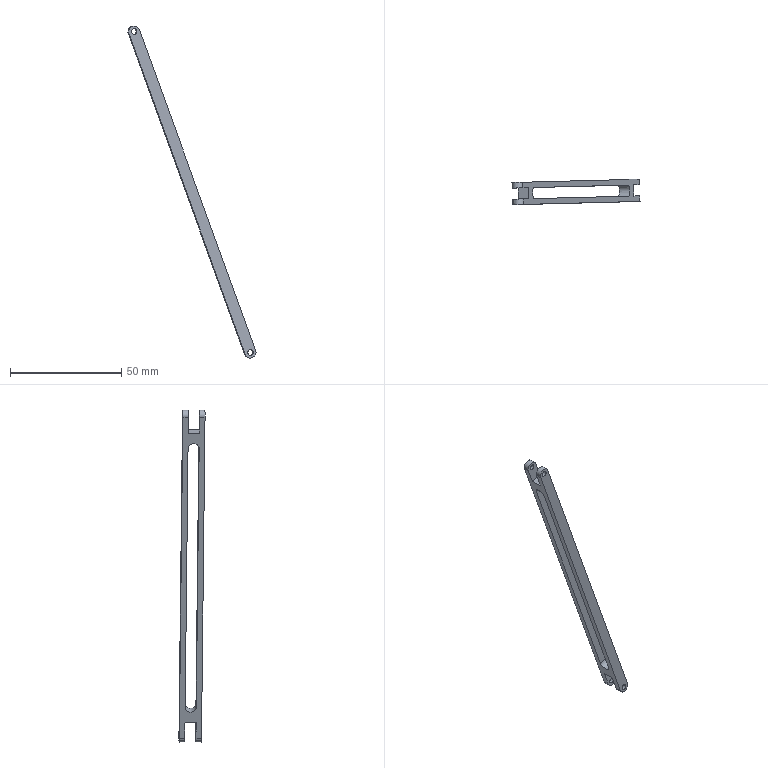Part | SolidWorks | features ICE 4, HoleWzd 2, Extrusion 1 | 1 solid | 29 faces | box 57.658 x 11.753 x 149.475 mm | volume 4168 mm3 | cylinder 17 | plane 12 | commonest cylinder face diameters 5 x9 2.5 x8
STEP:
#1=CARTESIAN_POINT('',(124.299,11.498,-265.344));
#2=VERTEX_POINT('',#1);
#3=CARTESIAN_POINT('',(121.801,11.422,-265.344));
#4=VERTEX_POINT('',#3);
#5=CARTESIAN_POINT('',(123.05,11.46,-265.344));
#6=DIRECTION('',(-0.03063,0.9995,0.));
#7=DIRECTION('',(-0.9995,-0.03063,0.));
#8=AXIS2_PLACEMENT_3D('',#5,#6,#7);
#9=CIRCLE('',#8,1.25);
#10=EDGE_CURVE('',#2,#4,#9,.T.);
#11=ORIENTED_EDGE('',*,*,#10,.F.);
#12=CARTESIAN_POINT('',(124.223,13.997,-265.344));
#13=VERTEX_POINT('',#12);
#14=CARTESIAN_POINT('',(124.223,13.997,-265.344));
#15=DIRECTION('',(-0.03063,0.9995,0.));
#16=VECTOR('',#15,1000.);
#17=LINE('',#14,#16);
#18=EDGE_CURVE('',#2,#13,#17,.T.);
#19=ORIENTED_EDGE('',*,*,#18,.T.);
#20=CARTESIAN_POINT('',(121.724,13.92,-265.344));
#21=VERTEX_POINT('',#20);
#22=CARTESIAN_POINT('',(122.973,13.959,-265.344));
#23=DIRECTION('',(-0.03063,0.9995,0.));
#24=DIRECTION('',(-0.9995,-0.03063,0.));
#25=AXIS2_PLACEMENT_3D('',#22,#23,#24);
#26=CIRCLE('',#25,1.25);
#27=EDGE_CURVE('',#13,#21,#26,.T.);
#28=ORIENTED_EDGE('',*,*,#27,.T.);
#29=CARTESIAN_POINT('',(121.724,13.92,-265.344));
#30=DIRECTION('',(-0.03063,0.9995,0.));
#31=VECTOR('',#30,1000.);
#32=LINE('',#29,#31);
#33=EDGE_CURVE('',#4,#21,#32,.T.);
#34=ORIENTED_EDGE('',*,*,#33,.F.);
#35=EDGE_LOOP('',(#11,#19,#28,#34));
#36=FACE_OUTER_BOUND('',#35,.T.);
#37=CARTESIAN_POINT('',(122.973,13.959,-265.344));
#38=DIRECTION('',(-0.03063,0.9995,0.));
#39=DIRECTION('',(-0.9995,-0.03063,0.));
#40=AXIS2_PLACEMENT_3D('',#37,#38,#39);
#41=CYLINDRICAL_SURFACE('',#40,1.25);
#42=ADVANCED_FACE('',(#36),#41,.F.);
#43=CARTESIAN_POINT('',(71.945,9.894,-120.869));
#44=VERTEX_POINT('',#43);
#45=CARTESIAN_POINT('',(69.447,9.817,-120.869));
#46=VERTEX_POINT('',#45);
#47=CARTESIAN_POINT('',(70.696,9.855,-120.869));
#48=DIRECTION('',(-0.03063,0.9995,0.));
#49=DIRECTION('',(-0.9995,-0.03063,0.));
#50=AXIS2_PLACEMENT_3D('',#47,#48,#49);
#51=CIRCLE('',#50,1.25);
#52=EDGE_CURVE('',#44,#46,#51,.T.);
#53=ORIENTED_EDGE('',*,*,#52,.F.);
#54=CARTESIAN_POINT('',(71.869,12.392,-120.869));
#55=VERTEX_POINT('',#54);
#56=CARTESIAN_POINT('',(71.869,12.392,-120.869));
#57=DIRECTION('',(-0.03063,0.9995,0.));
#58=VECTOR('',#57,1000.);
#59=LINE('',#56,#58);
#60=EDGE_CURVE('',#44,#55,#59,.T.);
#61=ORIENTED_EDGE('',*,*,#60,.T.);
#62=CARTESIAN_POINT('',(69.37,12.316,-120.869));
#63=VERTEX_POINT('',#62);
#64=CARTESIAN_POINT('',(70.619,12.354,-120.869));
#65=DIRECTION('',(-0.03063,0.9995,0.));
#66=DIRECTION('',(-0.9995,-0.03063,0.));
#67=AXIS2_PLACEMENT_3D('',#64,#65,#66);
#68=CIRCLE('',#67,1.25);
#69=EDGE_CURVE('',#55,#63,#68,.T.);
#70=ORIENTED_EDGE('',*,*,#69,.T.);
#71=CARTESIAN_POINT('',(69.37,12.316,-120.869));
#72=DIRECTION('',(-0.03063,0.9995,0.));
#73=VECTOR('',#72,1000.);
#74=LINE('',#71,#73);
#75=EDGE_CURVE('',#46,#63,#74,.T.);
#76=ORIENTED_EDGE('',*,*,#75,.F.);
#77=EDGE_LOOP('',(#53,#61,#70,#76));
#78=FACE_OUTER_BOUND('',#77,.T.);
#79=CARTESIAN_POINT('',(70.619,12.354,-120.869));
#80=DIRECTION('',(-0.03063,0.9995,0.));
#81=DIRECTION('',(-0.9995,-0.03063,0.));
#82=AXIS2_PLACEMENT_3D('',#79,#80,#81);
#83=CYLINDRICAL_SURFACE('',#82,1.25);
#84=ADVANCED_FACE('',(#78),#83,.F.);
#85=CARTESIAN_POINT('',(122.03,3.925,-265.344));
#86=VERTEX_POINT('',#85);
#87=CARTESIAN_POINT('',(124.529,4.002,-265.344));
#88=VERTEX_POINT('',#87);
#89=CARTESIAN_POINT('',(123.28,3.963,-265.344));
#90=DIRECTION('',(0.03063,-0.9995,0.));
#91=DIRECTION('',(0.9995,0.03063,0.));
#92=AXIS2_PLACEMENT_3D('',#89,#90,#91);
#93=CIRCLE('',#92,1.25);
#94=EDGE_CURVE('',#86,#88,#93,.T.);
#95=ORIENTED_EDGE('',*,*,#94,.T.);
#96=CARTESIAN_POINT('',(124.453,6.501,-265.344));
#97=VERTEX_POINT('',#96);
#98=CARTESIAN_POINT('',(124.453,6.501,-265.344));
#99=DIRECTION('',(-0.03063,0.9995,0.));
#100=VECTOR('',#99,1000.);
#101=LINE('',#98,#100);
#102=EDGE_CURVE('',#88,#97,#101,.T.);
#103=ORIENTED_EDGE('',*,*,#102,.T.);
#104=CARTESIAN_POINT('',(121.954,6.424,-265.344));
#105=VERTEX_POINT('',#104);
#106=CARTESIAN_POINT('',(123.203,6.462,-265.344));
#107=DIRECTION('',(-0.03063,0.9995,0.));
#108=DIRECTION('',(-0.9995,-0.03063,0.));
#109=AXIS2_PLACEMENT_3D('',#106,#107,#108);
#110=CIRCLE('',#109,1.25);
#111=EDGE_CURVE('',#97,#105,#110,.T.);
#112=ORIENTED_EDGE('',*,*,#111,.T.);
#113=CARTESIAN_POINT('',(121.954,6.424,-265.344));
#114=DIRECTION('',(-0.03063,0.9995,0.));
#115=VECTOR('',#114,1000.);
#116=LINE('',#113,#115);
#117=EDGE_CURVE('',#86,#105,#116,.T.);
#118=ORIENTED_EDGE('',*,*,#117,.F.);
#119=EDGE_LOOP('',(#95,#103,#112,#118));
#120=FACE_OUTER_BOUND('',#119,.T.);
#121=CARTESIAN_POINT('',(123.203,6.462,-265.344));
#122=DIRECTION('',(-0.03063,0.9995,0.));
#123=DIRECTION('',(-0.9995,-0.03063,0.));
#124=AXIS2_PLACEMENT_3D('',#121,#122,#123);
#125=CYLINDRICAL_SURFACE('',#124,1.25);
#126=ADVANCED_FACE('',(#120),#125,.F.);
#127=CARTESIAN_POINT('',(69.676,2.321,-120.869));
#128=VERTEX_POINT('',#127);
#129=CARTESIAN_POINT('',(72.175,2.397,-120.869));
#130=VERTEX_POINT('',#129);
#131=CARTESIAN_POINT('',(70.926,2.359,-120.869));
#132=DIRECTION('',(0.03063,-0.9995,0.));
#133=DIRECTION('',(0.9995,0.03063,0.));
#134=AXIS2_PLACEMENT_3D('',#131,#132,#133);
#135=CIRCLE('',#134,1.25);
#136=EDGE_CURVE('',#128,#130,#135,.T.);
#137=ORIENTED_EDGE('',*,*,#136,.T.);
#138=CARTESIAN_POINT('',(72.099,4.896,-120.869));
#139=VERTEX_POINT('',#138);
#140=CARTESIAN_POINT('',(72.099,4.896,-120.869));
#141=DIRECTION('',(-0.03063,0.9995,0.));
#142=VECTOR('',#141,1000.);
#143=LINE('',#140,#142);
#144=EDGE_CURVE('',#130,#139,#143,.T.);
#145=ORIENTED_EDGE('',*,*,#144,.T.);
#146=CARTESIAN_POINT('',(69.6,4.819,-120.869));
#147=VERTEX_POINT('',#146);
#148=CARTESIAN_POINT('',(70.849,4.858,-120.869));
#149=DIRECTION('',(-0.03063,0.9995,0.));
#150=DIRECTION('',(-0.9995,-0.03063,0.));
#151=AXIS2_PLACEMENT_3D('',#148,#149,#150);
#152=CIRCLE('',#151,1.25);
#153=EDGE_CURVE('',#139,#147,#152,.T.);
#154=ORIENTED_EDGE('',*,*,#153,.T.);
#155=CARTESIAN_POINT('',(69.6,4.819,-120.869));
#156=DIRECTION('',(-0.03063,0.9995,0.));
#157=VECTOR('',#156,1000.);
#158=LINE('',#155,#157);
#159=EDGE_CURVE('',#128,#147,#158,.T.);
#160=ORIENTED_EDGE('',*,*,#159,.F.);
#161=EDGE_LOOP('',(#137,#145,#154,#160));
#162=FACE_OUTER_BOUND('',#161,.T.);
#163=CARTESIAN_POINT('',(70.849,4.858,-120.869));
#164=DIRECTION('',(-0.03063,0.9995,0.));
#165=DIRECTION('',(-0.9995,-0.03063,0.));
#166=AXIS2_PLACEMENT_3D('',#163,#164,#165);
#167=CYLINDRICAL_SURFACE('',#166,1.25);
#168=ADVANCED_FACE('',(#162),#167,.F.);
#169=CARTESIAN_POINT('',(78.155,10.084,-134.119));
#170=VERTEX_POINT('',#169);
#171=CARTESIAN_POINT('',(77.38,7.585,-131.769));
#172=VERTEX_POINT('',#171);
#173=CARTESIAN_POINT('',(78.232,7.585,-134.119));
#174=DIRECTION('',(0.9397,0.0288,0.3408));
#175=DIRECTION('',(0.341,0.,-0.9401));
#176=AXIS2_PLACEMENT_3D('',#173,#174,#175);
#177=CIRCLE('',#176,2.5);
#178=EDGE_CURVE('',#170,#172,#177,.T.);
#179=ORIENTED_EDGE('',*,*,#178,.T.);
#180=CARTESIAN_POINT('',(72.681,7.441,-133.473));
#181=VERTEX_POINT('',#180);
#182=CARTESIAN_POINT('',(124.582,9.032,-114.647));
#183=DIRECTION('',(-0.9397,-0.0288,-0.3408));
#184=VECTOR('',#183,1000.);
#185=LINE('',#182,#184);
#186=EDGE_CURVE('',#172,#181,#185,.T.);
#187=ORIENTED_EDGE('',*,*,#186,.T.);
#188=CARTESIAN_POINT('',(73.457,9.94,-135.823));
#189=VERTEX_POINT('',#188);
#190=CARTESIAN_POINT('',(73.534,7.441,-135.823));
#191=DIRECTION('',(-0.9397,-0.0288,-0.3408));
#192=DIRECTION('',(-0.341,0.,0.9401));
#193=AXIS2_PLACEMENT_3D('',#190,#191,#192);
#194=CIRCLE('',#193,2.5);
#195=EDGE_CURVE('',#181,#189,#194,.T.);
#196=ORIENTED_EDGE('',*,*,#195,.T.);
#197=CARTESIAN_POINT('',(125.358,11.531,-116.998));
#198=DIRECTION('',(-0.9397,-0.0288,-0.3408));
#199=VECTOR('',#198,1000.);
#200=LINE('',#197,#199);
#201=EDGE_CURVE('',#170,#189,#200,.T.);
#202=ORIENTED_EDGE('',*,*,#201,.F.);
#203=EDGE_LOOP('',(#179,#187,#196,#202));
#204=FACE_OUTER_BOUND('',#203,.T.);
#205=CARTESIAN_POINT('',(125.435,9.032,-116.998));
#206=DIRECTION('',(-0.9397,-0.0288,-0.3408));
#207=DIRECTION('',(-0.341,0.,0.9401));
#208=AXIS2_PLACEMENT_3D('',#205,#206,#207);
#209=CYLINDRICAL_SURFACE('',#208,2.5);
#210=ADVANCED_FACE('',(#204),#209,.F.);
#211=CARTESIAN_POINT('',(125.702,6.539,-265.344));
#212=VERTEX_POINT('',#211);
#213=CARTESIAN_POINT('',(120.854,6.39,-266.196));
#214=VERTEX_POINT('',#213);
#215=CARTESIAN_POINT('',(123.203,6.462,-265.344));
#216=DIRECTION('',(-0.03063,0.9995,0.));
#217=DIRECTION('',(0.9995,0.03063,0.));
#218=AXIS2_PLACEMENT_3D('',#215,#216,#217);
#219=CIRCLE('',#218,2.5);
#220=EDGE_CURVE('',#212,#214,#219,.T.);
#221=ORIENTED_EDGE('',*,*,#220,.F.);
#222=CARTESIAN_POINT('',(125.779,4.04,-265.344));
#223=VERTEX_POINT('',#222);
#224=CARTESIAN_POINT('',(125.472,14.035,-265.344));
#225=DIRECTION('',(0.03063,-0.9995,0.));
#226=VECTOR('',#225,1000.);
#227=LINE('',#224,#226);
#228=EDGE_CURVE('',#212,#223,#227,.T.);
#229=ORIENTED_EDGE('',*,*,#228,.T.);
#230=CARTESIAN_POINT('',(120.931,3.891,-266.196));
#231=VERTEX_POINT('',#230);
#232=CARTESIAN_POINT('',(123.28,3.963,-265.344));
#233=DIRECTION('',(0.03063,-0.9995,0.));
#234=DIRECTION('',(0.9995,0.03063,0.));
#235=AXIS2_PLACEMENT_3D('',#232,#233,#234);
#236=CIRCLE('',#235,2.5);
#237=EDGE_CURVE('',#231,#223,#236,.T.);
#238=ORIENTED_EDGE('',*,*,#237,.F.);
#239=CARTESIAN_POINT('',(120.624,13.887,-266.196));
#240=DIRECTION('',(0.03063,-0.9995,0.));
#241=VECTOR('',#240,1000.);
#242=LINE('',#239,#241);
#243=EDGE_CURVE('',#214,#231,#242,.T.);
#244=ORIENTED_EDGE('',*,*,#243,.F.);
#245=EDGE_LOOP('',(#221,#229,#238,#244));
#246=FACE_OUTER_BOUND('',#245,.T.);
#247=CARTESIAN_POINT('',(122.973,13.959,-265.344));
#248=DIRECTION('',(0.03063,-0.9995,0.));
#249=DIRECTION('',(0.9995,0.03063,0.));
#250=AXIS2_PLACEMENT_3D('',#247,#248,#249);
#251=CYLINDRICAL_SURFACE('',#250,2.5);
#252=ADVANCED_FACE('',(#246),#251,.T.);
#253=CARTESIAN_POINT('',(120.624,13.887,-266.196));
#254=VERTEX_POINT('',#253);
#255=CARTESIAN_POINT('',(125.472,14.035,-265.344));
#256=VERTEX_POINT('',#255);
#257=CARTESIAN_POINT('',(122.973,13.959,-265.344));
#258=DIRECTION('',(0.03063,-0.9995,0.));
#259=DIRECTION('',(0.9995,0.03063,0.));
#260=AXIS2_PLACEMENT_3D('',#257,#258,#259);
#261=CIRCLE('',#260,2.5);
#262=EDGE_CURVE('',#254,#256,#261,.T.);
#263=ORIENTED_EDGE('',*,*,#262,.T.);
#264=CARTESIAN_POINT('',(125.549,11.536,-265.344));
#265=VERTEX_POINT('',#264);
#266=CARTESIAN_POINT('',(125.472,14.035,-265.344));
#267=DIRECTION('',(0.03063,-0.9995,0.));
#268=VECTOR('',#267,1000.);
#269=LINE('',#266,#268);
#270=EDGE_CURVE('',#256,#265,#269,.T.);
#271=ORIENTED_EDGE('',*,*,#270,.T.);
#272=CARTESIAN_POINT('',(120.701,11.388,-266.196));
#273=VERTEX_POINT('',#272);
#274=CARTESIAN_POINT('',(123.05,11.46,-265.344));
#275=DIRECTION('',(0.03063,-0.9995,0.));
#276=DIRECTION('',(-0.9995,-0.03063,0.));
#277=AXIS2_PLACEMENT_3D('',#274,#275,#276);
#278=CIRCLE('',#277,2.5);
#279=EDGE_CURVE('',#273,#265,#278,.T.);
#280=ORIENTED_EDGE('',*,*,#279,.F.);
#281=CARTESIAN_POINT('',(120.624,13.887,-266.196));
#282=DIRECTION('',(0.03063,-0.9995,0.));
#283=VECTOR('',#282,1000.);
#284=LINE('',#281,#283);
#285=EDGE_CURVE('',#254,#273,#284,.T.);
#286=ORIENTED_EDGE('',*,*,#285,.F.);
#287=EDGE_LOOP('',(#263,#271,#280,#286));
#288=FACE_OUTER_BOUND('',#287,.T.);
#289=CARTESIAN_POINT('',(122.973,13.959,-265.344));
#290=DIRECTION('',(0.03063,-0.9995,0.));
#291=DIRECTION('',(0.9995,0.03063,0.));
#292=AXIS2_PLACEMENT_3D('',#289,#290,#291);
#293=CYLINDRICAL_SURFACE('',#292,2.5);
#294=ADVANCED_FACE('',(#288),#293,.T.);
#295=ORIENTED_EDGE('',*,*,#270,.F.);
#296=CARTESIAN_POINT('',(125.323,14.031,-264.492));
#297=VERTEX_POINT('',#296);
#298=CARTESIAN_POINT('',(122.973,13.959,-265.344));
#299=DIRECTION('',(0.03063,-0.9995,0.));
#300=DIRECTION('',(0.9995,0.03063,0.));
#301=AXIS2_PLACEMENT_3D('',#298,#299,#300);
#302=CIRCLE('',#301,2.5);
#303=EDGE_CURVE('',#256,#297,#302,.T.);
#304=ORIENTED_EDGE('',*,*,#303,.T.);
#305=CARTESIAN_POINT('',(125.399,11.532,-264.492));
#306=VERTEX_POINT('',#305);
#307=CARTESIAN_POINT('',(125.323,14.031,-264.492));
#308=DIRECTION('',(0.03063,-0.9995,0.));
#309=VECTOR('',#308,1000.);
#310=LINE('',#307,#309);
#311=EDGE_CURVE('',#297,#306,#310,.T.);
#312=ORIENTED_EDGE('',*,*,#311,.T.);
#313=CARTESIAN_POINT('',(123.05,11.46,-265.344));
#314=DIRECTION('',(0.03063,-0.9995,0.));
#315=DIRECTION('',(-0.9995,-0.03063,0.));
#316=AXIS2_PLACEMENT_3D('',#313,#314,#315);
#317=CIRCLE('',#316,2.5);
#318=EDGE_CURVE('',#265,#306,#317,.T.);
#319=ORIENTED_EDGE('',*,*,#318,.F.);
#320=EDGE_LOOP('',(#295,#304,#312,#319));
#321=FACE_OUTER_BOUND('',#320,.T.);
#322=CARTESIAN_POINT('',(122.973,13.959,-265.344));
#323=DIRECTION('',(0.03063,-0.9995,0.));
#324=DIRECTION('',(0.9995,0.03063,0.));
#325=AXIS2_PLACEMENT_3D('',#322,#323,#324);
#326=CYLINDRICAL_SURFACE('',#325,2.5);
#327=ADVANCED_FACE('',(#321),#326,.T.);
#328=CARTESIAN_POINT('',(68.5,4.786,-121.721));
#329=VERTEX_POINT('',#328);
#330=CARTESIAN_POINT('',(73.198,4.93,-120.017));
#331=VERTEX_POINT('',#330);
#332=CARTESIAN_POINT('',(70.849,4.858,-120.869));
#333=DIRECTION('',(-0.03063,0.9995,0.));
#334=DIRECTION('',(0.9995,0.03063,0.));
#335=AXIS2_PLACEMENT_3D('',#332,#333,#334);
#336=CIRCLE('',#335,2.5);
#337=EDGE_CURVE('',#329,#331,#336,.T.);
#338=ORIENTED_EDGE('',*,*,#337,.F.);
#339=CARTESIAN_POINT('',(68.577,2.287,-121.721));
#340=VERTEX_POINT('',#339);
#341=CARTESIAN_POINT('',(68.27,12.282,-121.721));
#342=DIRECTION('',(0.03063,-0.9995,0.));
#343=VECTOR('',#342,1000.);
#344=LINE('',#341,#343);
#345=EDGE_CURVE('',#329,#340,#344,.T.);
#346=ORIENTED_EDGE('',*,*,#345,.T.);
#347=CARTESIAN_POINT('',(73.275,2.431,-120.017));
#348=VERTEX_POINT('',#347);
#349=CARTESIAN_POINT('',(70.926,2.359,-120.869));
#350=DIRECTION('',(0.03063,-0.9995,0.));
#351=DIRECTION('',(0.9995,0.03063,0.));
#352=AXIS2_PLACEMENT_3D('',#349,#350,#351);
#353=CIRCLE('',#352,2.5);
#354=EDGE_CURVE('',#348,#340,#353,.T.);
#355=ORIENTED_EDGE('',*,*,#354,.F.);
#356=CARTESIAN_POINT('',(72.969,12.426,-120.017));
#357=DIRECTION('',(0.03063,-0.9995,0.));
#358=VECTOR('',#357,1000.);
#359=LINE('',#356,#358);
#360=EDGE_CURVE('',#331,#348,#359,.T.);
#361=ORIENTED_EDGE('',*,*,#360,.F.);
#362=EDGE_LOOP('',(#338,#346,#355,#361));
#363=FACE_OUTER_BOUND('',#362,.T.);
#364=CARTESIAN_POINT('',(70.619,12.354,-120.869));
#365=DIRECTION('',(0.03063,-0.9995,0.));
#366=DIRECTION('',(0.9995,0.03063,0.));
#367=AXIS2_PLACEMENT_3D('',#364,#365,#366);
#368=CYLINDRICAL_SURFACE('',#367,2.5);
#369=ADVANCED_FACE('',(#363),#368,.T.);
#370=CARTESIAN_POINT('',(71.055,4.864,-128.772));
#371=VERTEX_POINT('',#370);
#372=CARTESIAN_POINT('',(71.055,4.864,-128.772));
#373=DIRECTION('',(-0.3407,-0.01044,0.9401));
#374=VECTOR('',#373,1000.);
#375=LINE('',#372,#374);
#376=EDGE_CURVE('',#371,#329,#375,.T.);
#377=ORIENTED_EDGE('',*,*,#376,.T.);
#378=ORIENTED_EDGE('',*,*,#337,.T.);
#379=CARTESIAN_POINT('',(75.753,5.008,-127.068));
#380=VERTEX_POINT('',#379);
#381=CARTESIAN_POINT('',(125.552,6.534,-264.492));
#382=DIRECTION('',(0.3407,0.01044,-0.9401));
#383=VECTOR('',#382,1000.);
#384=LINE('',#381,#383);
#385=EDGE_CURVE('',#331,#380,#384,.T.);
#386=ORIENTED_EDGE('',*,*,#385,.T.);
#387=CARTESIAN_POINT('',(122.956,6.455,-109.947));
#388=DIRECTION('',(-0.9397,-0.0288,-0.3408));
#389=VECTOR('',#388,1000.);
#390=LINE('',#387,#389);
#391=EDGE_CURVE('',#380,#371,#390,.T.);
#392=ORIENTED_EDGE('',*,*,#391,.T.);
#393=EDGE_LOOP('',(#377,#378,#386,#392));
#394=FACE_OUTER_BOUND('',#393,.T.);
#395=CARTESIAN_POINT('',(70.849,4.858,-120.869));
#396=DIRECTION('',(-0.03063,0.9995,0.));
#397=DIRECTION('',(-0.9995,-0.03063,0.));
#398=AXIS2_PLACEMENT_3D('',#395,#396,#397);
#399=CIRCLE('',#398,1.25);
#400=EDGE_CURVE('',#147,#139,#399,.T.);
#401=ORIENTED_EDGE('',*,*,#400,.F.);
#402=ORIENTED_EDGE('',*,*,#153,.F.);
#403=EDGE_LOOP('',(#401,#402));
#404=FACE_BOUND('',#403,.T.);
#405=CARTESIAN_POINT('',(122.956,6.455,-109.947));
#406=DIRECTION('',(0.03063,-0.9995,0.));
#407=DIRECTION('',(0.9995,0.03063,0.));
#408=AXIS2_PLACEMENT_3D('',#405,#406,#407);
#409=PLANE('',#408);
#410=ADVANCED_FACE('',(#394,#404),#409,.F.);
#411=ORIENTED_EDGE('',*,*,#228,.F.);
#412=CARTESIAN_POINT('',(125.552,6.534,-264.492));
#413=VERTEX_POINT('',#412);
#414=CARTESIAN_POINT('',(123.203,6.462,-265.344));
#415=DIRECTION('',(-0.03063,0.9995,0.));
#416=DIRECTION('',(0.9995,0.03063,0.));
#417=AXIS2_PLACEMENT_3D('',#414,#415,#416);
#418=CIRCLE('',#417,2.5);
#419=EDGE_CURVE('',#413,#212,#418,.T.);
#420=ORIENTED_EDGE('',*,*,#419,.F.);
#421=CARTESIAN_POINT('',(125.629,4.035,-264.492));
#422=VERTEX_POINT('',#421);
#423=CARTESIAN_POINT('',(125.323,14.031,-264.492));
#424=DIRECTION('',(0.03063,-0.9995,0.));
#425=VECTOR('',#424,1000.);
#426=LINE('',#423,#425);
#427=EDGE_CURVE('',#413,#422,#426,.T.);
#428=ORIENTED_EDGE('',*,*,#427,.T.);
#429=CARTESIAN_POINT('',(123.28,3.963,-265.344));
#430=DIRECTION('',(0.03063,-0.9995,0.));
#431=DIRECTION('',(0.9995,0.03063,0.));
#432=AXIS2_PLACEMENT_3D('',#429,#430,#431);
#433=CIRCLE('',#432,2.5);
#434=EDGE_CURVE('',#223,#422,#433,.T.);
#435=ORIENTED_EDGE('',*,*,#434,.F.);
#436=EDGE_LOOP('',(#411,#420,#428,#435));
#437=FACE_OUTER_BOUND('',#436,.T.);
#438=CARTESIAN_POINT('',(122.973,13.959,-265.344));
#439=DIRECTION('',(0.03063,-0.9995,0.));
#440=DIRECTION('',(0.9995,0.03063,0.));
#441=AXIS2_PLACEMENT_3D('',#438,#439,#440);
#442=CYLINDRICAL_SURFACE('',#441,2.5);
#443=ADVANCED_FACE('',(#437),#442,.T.);
#444=CARTESIAN_POINT('',(115.591,11.231,-252.094));
#445=VERTEX_POINT('',#444);
#446=CARTESIAN_POINT('',(115.744,6.234,-252.094));
#447=VERTEX_POINT('',#446);
#448=CARTESIAN_POINT('',(115.667,8.732,-252.094));
#449=DIRECTION('',(-0.9397,-0.0288,-0.3408));
#450=DIRECTION('',(-0.341,0.,0.9401));
#451=AXIS2_PLACEMENT_3D('',#448,#449,#450);
#452=CIRCLE('',#451,2.5);
#453=EDGE_CURVE('',#445,#447,#452,.T.);
#454=ORIENTED_EDGE('',*,*,#453,.F.);
#455=CARTESIAN_POINT('',(73.457,9.94,-135.823));
#456=DIRECTION('',(0.3407,0.01044,-0.9401));
#457=VECTOR('',#456,1000.);
#458=LINE('',#455,#457);
#459=EDGE_CURVE('',#189,#445,#458,.T.);
#460=ORIENTED_EDGE('',*,*,#459,.F.);
#461=ORIENTED_EDGE('',*,*,#195,.F.);
#462=CARTESIAN_POINT('',(73.61,4.942,-135.823));
#463=VERTEX_POINT('',#462);
#464=CARTESIAN_POINT('',(73.534,7.441,-135.823));
#465=DIRECTION('',(-0.9397,-0.0288,-0.3408));
#466=DIRECTION('',(-0.341,0.,0.9401));
#467=AXIS2_PLACEMENT_3D('',#464,#465,#466);
#468=CIRCLE('',#467,2.5);
#469=EDGE_CURVE('',#463,#181,#468,.T.);
#470=ORIENTED_EDGE('',*,*,#469,.F.);
#471=CARTESIAN_POINT('',(115.744,6.234,-252.094));
#472=DIRECTION('',(-0.3407,-0.01044,0.9401));
#473=VECTOR('',#472,1000.);
#474=LINE('',#471,#473);
#475=EDGE_CURVE('',#447,#463,#474,.T.);
#476=ORIENTED_EDGE('',*,*,#475,.F.);
#477=EDGE_LOOP('',(#454,#460,#461,#470,#476));
#478=FACE_BOUND('',#477,.T.);
#479=CARTESIAN_POINT('',(118.146,11.31,-259.145));
#480=VERTEX_POINT('',#479);
#481=CARTESIAN_POINT('',(118.146,11.31,-259.145));
#482=DIRECTION('',(0.3407,0.01044,-0.9401));
#483=VECTOR('',#482,1000.);
#484=LINE('',#481,#483);
#485=EDGE_CURVE('',#480,#273,#484,.T.);
#486=ORIENTED_EDGE('',*,*,#485,.F.);
#487=CARTESIAN_POINT('',(118.299,6.312,-259.145));
#488=VERTEX_POINT('',#487);
#489=CARTESIAN_POINT('',(118.299,6.312,-259.145));
#490=DIRECTION('',(-0.03063,0.9995,0.));
#491=VECTOR('',#490,1000.);
#492=LINE('',#489,#491);
#493=EDGE_CURVE('',#488,#480,#492,.T.);
#494=ORIENTED_EDGE('',*,*,#493,.F.);
#495=CARTESIAN_POINT('',(120.854,6.39,-266.196));
#496=DIRECTION('',(-0.3407,-0.01044,0.9401));
#497=VECTOR('',#496,1000.);
#498=LINE('',#495,#497);
#499=EDGE_CURVE('',#214,#488,#498,.T.);
#500=ORIENTED_EDGE('',*,*,#499,.F.);
#501=ORIENTED_EDGE('',*,*,#243,.T.);
#502=CARTESIAN_POINT('',(68.577,2.287,-121.721));
#503=DIRECTION('',(0.3407,0.01044,-0.9401));
#504=VECTOR('',#503,1000.);
#505=LINE('',#502,#504);
#506=EDGE_CURVE('',#340,#231,#505,.T.);
#507=ORIENTED_EDGE('',*,*,#506,.F.);
#508=ORIENTED_EDGE('',*,*,#345,.F.);
#509=ORIENTED_EDGE('',*,*,#376,.F.);
#510=CARTESIAN_POINT('',(70.902,9.862,-128.772));
#511=VERTEX_POINT('',#510);
#512=CARTESIAN_POINT('',(70.902,9.862,-128.772));
#513=DIRECTION('',(0.03063,-0.9995,0.));
#514=VECTOR('',#513,1000.);
#515=LINE('',#512,#514);
#516=EDGE_CURVE('',#511,#371,#515,.T.);
#517=ORIENTED_EDGE('',*,*,#516,.F.);
#518=CARTESIAN_POINT('',(68.347,9.783,-121.721));
#519=VERTEX_POINT('',#518);
#520=CARTESIAN_POINT('',(68.347,9.783,-121.721));
#521=DIRECTION('',(0.3407,0.01044,-0.9401));
#522=VECTOR('',#521,1000.);
#523=LINE('',#520,#522);
#524=EDGE_CURVE('',#519,#511,#523,.T.);
#525=ORIENTED_EDGE('',*,*,#524,.F.);
#526=CARTESIAN_POINT('',(68.27,12.282,-121.721));
#527=VERTEX_POINT('',#526);
#528=CARTESIAN_POINT('',(68.27,12.282,-121.721));
#529=DIRECTION('',(0.03063,-0.9995,0.));
#530=VECTOR('',#529,1000.);
#531=LINE('',#528,#530);
#532=EDGE_CURVE('',#527,#519,#531,.T.);
#533=ORIENTED_EDGE('',*,*,#532,.F.);
#534=CARTESIAN_POINT('',(68.27,12.282,-121.721));
#535=DIRECTION('',(0.3407,0.01044,-0.9401));
#536=VECTOR('',#535,1000.);
#537=LINE('',#534,#536);
#538=EDGE_CURVE('',#527,#254,#537,.T.);
#539=ORIENTED_EDGE('',*,*,#538,.T.);
#540=ORIENTED_EDGE('',*,*,#285,.T.);
#541=EDGE_LOOP('',(#486,#494,#500,#501,#507,#508,#509,#517,#525,#533,#539,#540));
#542=FACE_OUTER_BOUND('',#541,.T.);
#543=CARTESIAN_POINT('',(68.27,12.282,-121.721));
#544=DIRECTION('',(-0.9397,-0.0288,-0.3408));
#545=DIRECTION('',(-0.341,0.,0.9401));
#546=AXIS2_PLACEMENT_3D('',#543,#544,#545);
#547=PLANE('',#546);
#548=ADVANCED_FACE('',(#478,#542),#547,.T.);
#549=CARTESIAN_POINT('',(73.045,9.927,-120.017));
#550=VERTEX_POINT('',#549);
#551=CARTESIAN_POINT('',(70.696,9.855,-120.869));
#552=DIRECTION('',(0.03063,-0.9995,0.));
#553=DIRECTION('',(-0.9995,-0.03063,0.));
#554=AXIS2_PLACEMENT_3D('',#551,#552,#553);
#555=CIRCLE('',#554,2.5);
#556=EDGE_CURVE('',#550,#519,#555,.T.);
#557=ORIENTED_EDGE('',*,*,#556,.F.);
#558=CARTESIAN_POINT('',(72.969,12.426,-120.017));
#559=VERTEX_POINT('',#558);
#560=CARTESIAN_POINT('',(72.969,12.426,-120.017));
#561=DIRECTION('',(0.03063,-0.9995,0.));
#562=VECTOR('',#561,1000.);
#563=LINE('',#560,#562);
#564=EDGE_CURVE('',#559,#550,#563,.T.);
#565=ORIENTED_EDGE('',*,*,#564,.F.);
#566=CARTESIAN_POINT('',(70.619,12.354,-120.869));
#567=DIRECTION('',(0.03063,-0.9995,0.));
#568=DIRECTION('',(0.9995,0.03063,0.));
#569=AXIS2_PLACEMENT_3D('',#566,#567,#568);
#570=CIRCLE('',#569,2.5);
#571=EDGE_CURVE('',#559,#527,#570,.T.);
#572=ORIENTED_EDGE('',*,*,#571,.T.);
#573=ORIENTED_EDGE('',*,*,#532,.T.);
#574=EDGE_LOOP('',(#557,#565,#572,#573));
#575=FACE_OUTER_BOUND('',#574,.T.);
#576=CARTESIAN_POINT('',(70.619,12.354,-120.869));
#577=DIRECTION('',(0.03063,-0.9995,0.));
#578=DIRECTION('',(0.9995,0.03063,0.));
#579=AXIS2_PLACEMENT_3D('',#576,#577,#578);
#580=CYLINDRICAL_SURFACE('',#579,2.5);
#581=ADVANCED_FACE('',(#575),#580,.T.);
#582=CARTESIAN_POINT('',(120.442,6.378,-250.39));
#583=VERTEX_POINT('',#582);
#584=CARTESIAN_POINT('',(120.289,11.375,-250.39));
#585=VERTEX_POINT('',#584);
#586=CARTESIAN_POINT('',(120.366,8.876,-250.39));
#587=DIRECTION('',(0.9397,0.0288,0.3408));
#588=DIRECTION('',(0.341,0.,-0.9401));
#589=AXIS2_PLACEMENT_3D('',#586,#587,#588);
#590=CIRCLE('',#589,2.5);
#591=EDGE_CURVE('',#583,#585,#590,.T.);
#592=ORIENTED_EDGE('',*,*,#591,.F.);
#593=CARTESIAN_POINT('',(78.309,5.086,-134.119));
#594=VERTEX_POINT('',#593);
#595=CARTESIAN_POINT('',(125.552,6.534,-264.492));
#596=DIRECTION('',(0.3407,0.01044,-0.9401));
#597=VECTOR('',#596,1000.);
#598=LINE('',#595,#597);
#599=EDGE_CURVE('',#594,#583,#598,.T.);
#600=ORIENTED_EDGE('',*,*,#599,.F.);
#601=CARTESIAN_POINT('',(78.232,7.585,-134.119));
#602=DIRECTION('',(0.9397,0.0288,0.3408));
#603=DIRECTION('',(0.341,0.,-0.9401));
#604=AXIS2_PLACEMENT_3D('',#601,#602,#603);
#605=CIRCLE('',#604,2.5);
#606=EDGE_CURVE('',#172,#594,#605,.T.);
#607=ORIENTED_EDGE('',*,*,#606,.F.);
#608=ORIENTED_EDGE('',*,*,#178,.F.);
#609=CARTESIAN_POINT('',(125.399,11.532,-264.492));
#610=DIRECTION('',(-0.3407,-0.01044,0.9401));
#611=VECTOR('',#610,1000.);
#612=LINE('',#609,#611);
#613=EDGE_CURVE('',#585,#170,#612,.T.);
#614=ORIENTED_EDGE('',*,*,#613,.F.);
#615=EDGE_LOOP('',(#592,#600,#607,#608,#614));
#616=FACE_BOUND('',#615,.T.);
#617=CARTESIAN_POINT('',(122.844,11.454,-257.441));
#618=VERTEX_POINT('',#617);
#619=CARTESIAN_POINT('',(125.399,11.532,-264.492));
#620=DIRECTION('',(-0.3407,-0.01044,0.9401));
#621=VECTOR('',#620,1000.);
#622=LINE('',#619,#621);
#623=EDGE_CURVE('',#306,#618,#622,.T.);
#624=ORIENTED_EDGE('',*,*,#623,.F.);
#625=ORIENTED_EDGE('',*,*,#311,.F.);
#626=CARTESIAN_POINT('',(125.323,14.031,-264.492));
#627=DIRECTION('',(-0.3407,-0.01044,0.9401));
#628=VECTOR('',#627,1000.);
#629=LINE('',#626,#628);
#630=EDGE_CURVE('',#297,#559,#629,.T.);
#631=ORIENTED_EDGE('',*,*,#630,.T.);
#632=ORIENTED_EDGE('',*,*,#564,.T.);
#633=CARTESIAN_POINT('',(75.6,10.006,-127.068));
#634=VERTEX_POINT('',#633);
#635=CARTESIAN_POINT('',(125.399,11.532,-264.492));
#636=DIRECTION('',(-0.3407,-0.01044,0.9401));
#637=VECTOR('',#636,1000.);
#638=LINE('',#635,#637);
#639=EDGE_CURVE('',#634,#550,#638,.T.);
#640=ORIENTED_EDGE('',*,*,#639,.F.);
#641=CARTESIAN_POINT('',(75.524,12.504,-127.068));
#642=DIRECTION('',(-0.03063,0.9995,0.));
#643=VECTOR('',#642,1000.);
#644=LINE('',#641,#643);
#645=EDGE_CURVE('',#380,#634,#644,.T.);
#646=ORIENTED_EDGE('',*,*,#645,.F.);
#647=ORIENTED_EDGE('',*,*,#385,.F.);
#648=ORIENTED_EDGE('',*,*,#360,.T.);
#649=CARTESIAN_POINT('',(125.629,4.035,-264.492));
#650=DIRECTION('',(-0.3407,-0.01044,0.9401));
#651=VECTOR('',#650,1000.);
#652=LINE('',#649,#651);
#653=EDGE_CURVE('',#422,#348,#652,.T.);
#654=ORIENTED_EDGE('',*,*,#653,.F.);
#655=ORIENTED_EDGE('',*,*,#427,.F.);
#656=CARTESIAN_POINT('',(122.997,6.456,-257.441));
#657=VERTEX_POINT('',#656);
#658=CARTESIAN_POINT('',(125.552,6.534,-264.492));
#659=DIRECTION('',(0.3407,0.01044,-0.9401));
#660=VECTOR('',#659,1000.);
#661=LINE('',#658,#660);
#662=EDGE_CURVE('',#657,#413,#661,.T.);
#663=ORIENTED_EDGE('',*,*,#662,.F.);
#664=CARTESIAN_POINT('',(122.768,13.952,-257.441));
#665=DIRECTION('',(0.03063,-0.9995,0.));
#666=VECTOR('',#665,1000.);
#667=LINE('',#664,#666);
#668=EDGE_CURVE('',#618,#657,#667,.T.);
#669=ORIENTED_EDGE('',*,*,#668,.F.);
#670=EDGE_LOOP('',(#624,#625,#631,#632,#640,#646,#647,#648,#654,#655,#663,#669));
#671=FACE_OUTER_BOUND('',#670,.T.);
#672=CARTESIAN_POINT('',(125.323,14.031,-264.492));
#673=DIRECTION('',(0.9397,0.0288,0.3408));
#674=DIRECTION('',(0.341,0.,-0.9401));
#675=AXIS2_PLACEMENT_3D('',#672,#673,#674);
#676=PLANE('',#675);
#677=ADVANCED_FACE('',(#616,#671),#676,.T.);
#678=CARTESIAN_POINT('',(122.973,13.959,-265.344));
#679=DIRECTION('',(-0.03063,0.9995,0.));
#680=DIRECTION('',(-0.9995,-0.03063,0.));
#681=AXIS2_PLACEMENT_3D('',#678,#679,#680);
#682=CIRCLE('',#681,1.25);
#683=EDGE_CURVE('',#21,#13,#682,.T.);
#684=ORIENTED_EDGE('',*,*,#683,.F.);
#685=ORIENTED_EDGE('',*,*,#27,.F.);
#686=EDGE_LOOP('',(#684,#685));
#687=FACE_BOUND('',#686,.T.);
#688=CARTESIAN_POINT('',(70.619,12.354,-120.869));
#689=DIRECTION('',(-0.03063,0.9995,0.));
#690=DIRECTION('',(-0.9995,-0.03063,0.));
#691=AXIS2_PLACEMENT_3D('',#688,#689,#690);
#692=CIRCLE('',#691,1.25);
#693=EDGE_CURVE('',#63,#55,#692,.T.);
#694=ORIENTED_EDGE('',*,*,#693,.F.);
#695=ORIENTED_EDGE('',*,*,#69,.F.);
#696=EDGE_LOOP('',(#694,#695));
#697=FACE_BOUND('',#696,.T.);
#698=ORIENTED_EDGE('',*,*,#262,.F.);
#699=ORIENTED_EDGE('',*,*,#538,.F.);
#700=ORIENTED_EDGE('',*,*,#571,.F.);
#701=ORIENTED_EDGE('',*,*,#630,.F.);
#702=ORIENTED_EDGE('',*,*,#303,.F.);
#703=EDGE_LOOP('',(#698,#699,#700,#701,#702));
#704=FACE_OUTER_BOUND('',#703,.T.);
#705=CARTESIAN_POINT('',(122.973,13.959,-265.344));
#706=DIRECTION('',(0.03063,-0.9995,0.));
#707=DIRECTION('',(0.9995,0.03063,0.));
#708=AXIS2_PLACEMENT_3D('',#705,#706,#707);
#709=PLANE('',#708);
#710=ADVANCED_FACE('',(#687,#697,#704),#709,.F.);
#711=ORIENTED_EDGE('',*,*,#94,.F.);
#712=CARTESIAN_POINT('',(123.28,3.963,-265.344));
#713=DIRECTION('',(0.03063,-0.9995,0.));
#714=DIRECTION('',(0.9995,0.03063,0.));
#715=AXIS2_PLACEMENT_3D('',#712,#713,#714);
#716=CIRCLE('',#715,1.25);
#717=EDGE_CURVE('',#88,#86,#716,.T.);
#718=ORIENTED_EDGE('',*,*,#717,.F.);
#719=EDGE_LOOP('',(#711,#718));
#720=FACE_BOUND('',#719,.T.);
#721=ORIENTED_EDGE('',*,*,#136,.F.);
#722=CARTESIAN_POINT('',(70.926,2.359,-120.869));
#723=DIRECTION('',(0.03063,-0.9995,0.));
#724=DIRECTION('',(0.9995,0.03063,0.));
#725=AXIS2_PLACEMENT_3D('',#722,#723,#724);
#726=CIRCLE('',#725,1.25);
#727=EDGE_CURVE('',#130,#128,#726,.T.);
#728=ORIENTED_EDGE('',*,*,#727,.F.);
#729=EDGE_LOOP('',(#721,#728));
#730=FACE_BOUND('',#729,.T.);
#731=ORIENTED_EDGE('',*,*,#237,.T.);
#732=ORIENTED_EDGE('',*,*,#434,.T.);
#733=ORIENTED_EDGE('',*,*,#653,.T.);
#734=ORIENTED_EDGE('',*,*,#354,.T.);
#735=ORIENTED_EDGE('',*,*,#506,.T.);
#736=EDGE_LOOP('',(#731,#732,#733,#734,#735));
#737=FACE_OUTER_BOUND('',#736,.T.);
#738=CARTESIAN_POINT('',(123.28,3.963,-265.344));
#739=DIRECTION('',(0.03063,-0.9995,0.));
#740=DIRECTION('',(0.9995,0.03063,0.));
#741=AXIS2_PLACEMENT_3D('',#738,#739,#740);
#742=PLANE('',#741);
#743=ADVANCED_FACE('',(#720,#730,#737),#742,.T.);
#744=ORIENTED_EDGE('',*,*,#645,.T.);
#745=CARTESIAN_POINT('',(122.803,11.452,-109.947));
#746=DIRECTION('',(-0.9397,-0.0288,-0.3408));
#747=VECTOR('',#746,1000.);
#748=LINE('',#745,#747);
#749=EDGE_CURVE('',#634,#511,#748,.T.);
#750=ORIENTED_EDGE('',*,*,#749,.T.);
#751=ORIENTED_EDGE('',*,*,#516,.T.);
#752=ORIENTED_EDGE('',*,*,#391,.F.);
#753=EDGE_LOOP('',(#744,#750,#751,#752));
#754=FACE_OUTER_BOUND('',#753,.T.);
#755=CARTESIAN_POINT('',(122.803,11.452,-109.947));
#756=DIRECTION('',(0.3407,0.01044,-0.9401));
#757=DIRECTION('',(-0.9402,0.,-0.3407));
#758=AXIS2_PLACEMENT_3D('',#755,#756,#757);
#759=PLANE('',#758);
#760=ADVANCED_FACE('',(#754),#759,.F.);
#761=CARTESIAN_POINT('',(70.696,9.855,-120.869));
#762=DIRECTION('',(-0.03063,0.9995,0.));
#763=DIRECTION('',(-0.9995,-0.03063,0.));
#764=AXIS2_PLACEMENT_3D('',#761,#762,#763);
#765=CIRCLE('',#764,1.25);
#766=EDGE_CURVE('',#46,#44,#765,.T.);
#767=ORIENTED_EDGE('',*,*,#766,.T.);
#768=ORIENTED_EDGE('',*,*,#52,.T.);
#769=EDGE_LOOP('',(#767,#768));
#770=FACE_BOUND('',#769,.T.);
#771=ORIENTED_EDGE('',*,*,#639,.T.);
#772=ORIENTED_EDGE('',*,*,#556,.T.);
#773=ORIENTED_EDGE('',*,*,#524,.T.);
#774=ORIENTED_EDGE('',*,*,#749,.F.);
#775=EDGE_LOOP('',(#771,#772,#773,#774));
#776=FACE_OUTER_BOUND('',#775,.T.);
#777=CARTESIAN_POINT('',(120.248,11.374,-102.896));
#778=DIRECTION('',(-0.03063,0.9995,0.));
#779=DIRECTION('',(-0.9995,-0.03063,0.));
#780=AXIS2_PLACEMENT_3D('',#777,#778,#779);
#781=PLANE('',#780);
#782=ADVANCED_FACE('',(#770,#776),#781,.F.);
#783=ORIENTED_EDGE('',*,*,#485,.T.);
#784=ORIENTED_EDGE('',*,*,#279,.T.);
#785=ORIENTED_EDGE('',*,*,#318,.T.);
#786=ORIENTED_EDGE('',*,*,#623,.T.);
#787=CARTESIAN_POINT('',(170.047,12.9,-240.32));
#788=DIRECTION('',(-0.9397,-0.0288,-0.3408));
#789=VECTOR('',#788,1000.);
#790=LINE('',#787,#789);
#791=EDGE_CURVE('',#618,#480,#790,.T.);
#792=ORIENTED_EDGE('',*,*,#791,.T.);
#793=EDGE_LOOP('',(#783,#784,#785,#786,#792));
#794=FACE_OUTER_BOUND('',#793,.T.);
#795=CARTESIAN_POINT('',(123.05,11.46,-265.344));
#796=DIRECTION('',(-0.03063,0.9995,0.));
#797=DIRECTION('',(-0.9995,-0.03063,0.));
#798=AXIS2_PLACEMENT_3D('',#795,#796,#797);
#799=CIRCLE('',#798,1.25);
#800=EDGE_CURVE('',#4,#2,#799,.T.);
#801=ORIENTED_EDGE('',*,*,#800,.T.);
#802=ORIENTED_EDGE('',*,*,#10,.T.);
#803=EDGE_LOOP('',(#801,#802));
#804=FACE_BOUND('',#803,.T.);
#805=CARTESIAN_POINT('',(170.047,12.9,-240.32));
#806=DIRECTION('',(-0.03063,0.9995,0.));
#807=DIRECTION('',(-0.9995,-0.03063,0.));
#808=AXIS2_PLACEMENT_3D('',#805,#806,#807);
#809=PLANE('',#808);
#810=ADVANCED_FACE('',(#794,#804),#809,.F.);
#811=ORIENTED_EDGE('',*,*,#668,.T.);
#812=CARTESIAN_POINT('',(170.2,7.903,-240.32));
#813=DIRECTION('',(-0.9397,-0.0288,-0.3408));
#814=VECTOR('',#813,1000.);
#815=LINE('',#812,#814);
#816=EDGE_CURVE('',#657,#488,#815,.T.);
#817=ORIENTED_EDGE('',*,*,#816,.T.);
#818=ORIENTED_EDGE('',*,*,#493,.T.);
#819=ORIENTED_EDGE('',*,*,#791,.F.);
#820=EDGE_LOOP('',(#811,#817,#818,#819));
#821=FACE_OUTER_BOUND('',#820,.T.);
#822=CARTESIAN_POINT('',(170.2,7.903,-240.32));
#823=DIRECTION('',(-0.3407,-0.01044,0.9401));
#824=DIRECTION('',(0.9402,0.,0.3407));
#825=AXIS2_PLACEMENT_3D('',#822,#823,#824);
#826=PLANE('',#825);
#827=ADVANCED_FACE('',(#821),#826,.F.);
#828=CARTESIAN_POINT('',(123.203,6.462,-265.344));
#829=DIRECTION('',(-0.03063,0.9995,0.));
#830=DIRECTION('',(-0.9995,-0.03063,0.));
#831=AXIS2_PLACEMENT_3D('',#828,#829,#830);
#832=CIRCLE('',#831,1.25);
#833=EDGE_CURVE('',#105,#97,#832,.T.);
#834=ORIENTED_EDGE('',*,*,#833,.F.);
#835=ORIENTED_EDGE('',*,*,#111,.F.);
#836=EDGE_LOOP('',(#834,#835));
#837=FACE_BOUND('',#836,.T.);
#838=ORIENTED_EDGE('',*,*,#662,.T.);
#839=ORIENTED_EDGE('',*,*,#419,.T.);
#840=ORIENTED_EDGE('',*,*,#220,.T.);
#841=ORIENTED_EDGE('',*,*,#499,.T.);
#842=ORIENTED_EDGE('',*,*,#816,.F.);
#843=EDGE_LOOP('',(#838,#839,#840,#841,#842));
#844=FACE_OUTER_BOUND('',#843,.T.);
#845=CARTESIAN_POINT('',(172.755,7.981,-247.371));
#846=DIRECTION('',(0.03063,-0.9995,0.));
#847=DIRECTION('',(0.9995,0.03063,0.));
#848=AXIS2_PLACEMENT_3D('',#845,#846,#847);
#849=PLANE('',#848);
#850=ADVANCED_FACE('',(#837,#844),#849,.F.);
#851=ORIENTED_EDGE('',*,*,#591,.T.);
#852=CARTESIAN_POINT('',(167.492,12.822,-233.269));
#853=DIRECTION('',(-0.9397,-0.0288,-0.3408));
#854=VECTOR('',#853,1000.);
#855=LINE('',#852,#854);
#856=EDGE_CURVE('',#585,#445,#855,.T.);
#857=ORIENTED_EDGE('',*,*,#856,.T.);
#858=ORIENTED_EDGE('',*,*,#453,.T.);
#859=CARTESIAN_POINT('',(167.645,7.824,-233.269));
#860=DIRECTION('',(-0.9397,-0.0288,-0.3408));
#861=VECTOR('',#860,1000.);
#862=LINE('',#859,#861);
#863=EDGE_CURVE('',#583,#447,#862,.T.);
#864=ORIENTED_EDGE('',*,*,#863,.F.);
#865=EDGE_LOOP('',(#851,#857,#858,#864));
#866=FACE_OUTER_BOUND('',#865,.T.);
#867=CARTESIAN_POINT('',(167.568,10.323,-233.269));
#868=DIRECTION('',(-0.9397,-0.0288,-0.3408));
#869=DIRECTION('',(-0.341,0.,0.9401));
#870=AXIS2_PLACEMENT_3D('',#867,#868,#869);
#871=CYLINDRICAL_SURFACE('',#870,2.5);
#872=ADVANCED_FACE('',(#866),#871,.F.);
#873=ORIENTED_EDGE('',*,*,#613,.T.);
#874=ORIENTED_EDGE('',*,*,#201,.T.);
#875=ORIENTED_EDGE('',*,*,#459,.T.);
#876=ORIENTED_EDGE('',*,*,#856,.F.);
#877=EDGE_LOOP('',(#873,#874,#875,#876));
#878=FACE_OUTER_BOUND('',#877,.T.);
#879=CARTESIAN_POINT('',(125.358,11.531,-116.998));
#880=DIRECTION('',(-0.03063,0.9995,0.));
#881=DIRECTION('',(-0.9995,-0.03063,0.));
#882=AXIS2_PLACEMENT_3D('',#879,#880,#881);
#883=PLANE('',#882);
#884=ADVANCED_FACE('',(#878),#883,.F.);
#885=ORIENTED_EDGE('',*,*,#186,.F.);
#886=ORIENTED_EDGE('',*,*,#606,.T.);
#887=CARTESIAN_POINT('',(125.511,6.533,-116.998));
#888=DIRECTION('',(-0.9397,-0.0288,-0.3408));
#889=VECTOR('',#888,1000.);
#890=LINE('',#887,#889);
#891=EDGE_CURVE('',#594,#463,#890,.T.);
#892=ORIENTED_EDGE('',*,*,#891,.T.);
#893=ORIENTED_EDGE('',*,*,#469,.T.);
#894=EDGE_LOOP('',(#885,#886,#892,#893));
#895=FACE_OUTER_BOUND('',#894,.T.);
#896=CARTESIAN_POINT('',(125.435,9.032,-116.998));
#897=DIRECTION('',(-0.9397,-0.0288,-0.3408));
#898=DIRECTION('',(-0.341,0.,0.9401));
#899=AXIS2_PLACEMENT_3D('',#896,#897,#898);
#900=CYLINDRICAL_SURFACE('',#899,2.5);
#901=ADVANCED_FACE('',(#895),#900,.F.);
#902=ORIENTED_EDGE('',*,*,#599,.T.);
#903=ORIENTED_EDGE('',*,*,#863,.T.);
#904=ORIENTED_EDGE('',*,*,#475,.T.);
#905=ORIENTED_EDGE('',*,*,#891,.F.);
#906=EDGE_LOOP('',(#902,#903,#904,#905));
#907=FACE_OUTER_BOUND('',#906,.T.);
#908=CARTESIAN_POINT('',(167.645,7.824,-233.269));
#909=DIRECTION('',(0.03063,-0.9995,0.));
#910=DIRECTION('',(0.9995,0.03063,0.));
#911=AXIS2_PLACEMENT_3D('',#908,#909,#910);
#912=PLANE('',#911);
#913=ADVANCED_FACE('',(#907),#912,.F.);
#914=ORIENTED_EDGE('',*,*,#144,.F.);
#915=ORIENTED_EDGE('',*,*,#727,.T.);
#916=ORIENTED_EDGE('',*,*,#159,.T.);
#917=ORIENTED_EDGE('',*,*,#400,.T.);
#918=EDGE_LOOP('',(#914,#915,#916,#917));
#919=FACE_OUTER_BOUND('',#918,.T.);
#920=CARTESIAN_POINT('',(70.849,4.858,-120.869));
#921=DIRECTION('',(-0.03063,0.9995,0.));
#922=DIRECTION('',(-0.9995,-0.03063,0.));
#923=AXIS2_PLACEMENT_3D('',#920,#921,#922);
#924=CYLINDRICAL_SURFACE('',#923,1.25);
#925=ADVANCED_FACE('',(#919),#924,.F.);
#926=ORIENTED_EDGE('',*,*,#102,.F.);
#927=ORIENTED_EDGE('',*,*,#717,.T.);
#928=ORIENTED_EDGE('',*,*,#117,.T.);
#929=ORIENTED_EDGE('',*,*,#833,.T.);
#930=EDGE_LOOP('',(#926,#927,#928,#929));
#931=FACE_OUTER_BOUND('',#930,.T.);
#932=CARTESIAN_POINT('',(123.203,6.462,-265.344));
#933=DIRECTION('',(-0.03063,0.9995,0.));
#934=DIRECTION('',(-0.9995,-0.03063,0.));
#935=AXIS2_PLACEMENT_3D('',#932,#933,#934);
#936=CYLINDRICAL_SURFACE('',#935,1.25);
#937=ADVANCED_FACE('',(#931),#936,.F.);
#938=ORIENTED_EDGE('',*,*,#60,.F.);
#939=ORIENTED_EDGE('',*,*,#766,.F.);
#940=ORIENTED_EDGE('',*,*,#75,.T.);
#941=ORIENTED_EDGE('',*,*,#693,.T.);
#942=EDGE_LOOP('',(#938,#939,#940,#941));
#943=FACE_OUTER_BOUND('',#942,.T.);
#944=CARTESIAN_POINT('',(70.619,12.354,-120.869));
#945=DIRECTION('',(-0.03063,0.9995,0.));
#946=DIRECTION('',(-0.9995,-0.03063,0.));
#947=AXIS2_PLACEMENT_3D('',#944,#945,#946);
#948=CYLINDRICAL_SURFACE('',#947,1.25);
#949=ADVANCED_FACE('',(#943),#948,.F.);
#950=ORIENTED_EDGE('',*,*,#18,.F.);
#951=ORIENTED_EDGE('',*,*,#800,.F.);
#952=ORIENTED_EDGE('',*,*,#33,.T.);
#953=ORIENTED_EDGE('',*,*,#683,.T.);
#954=EDGE_LOOP('',(#950,#951,#952,#953));
#955=FACE_OUTER_BOUND('',#954,.T.);
#956=CARTESIAN_POINT('',(122.973,13.959,-265.344));
#957=DIRECTION('',(-0.03063,0.9995,0.));
#958=DIRECTION('',(-0.9995,-0.03063,0.));
#959=AXIS2_PLACEMENT_3D('',#956,#957,#958);
#960=CYLINDRICAL_SURFACE('',#959,1.25);
#961=ADVANCED_FACE('',(#955),#960,.F.);
#962=CLOSED_SHELL('',(#42,#84,#126,#168,#210,#252,#294,#327,#369,#410,#443,#548,#581,#677,#710,#743,#760,#782,#810,#827,#850,#872,#884,#901,#913,#925,#937,#949,#961));
#963=MANIFOLD_SOLID_BREP('',#962);
#964=CARTESIAN_POINT('',(0.,0.,0.));
#965=DIRECTION('',(0.,0.,1.));
#966=DIRECTION('',(1.,0.,0.));
#967=AXIS2_PLACEMENT_3D('',#964,#965,#966);
#968=(LENGTH_UNIT()NAMED_UNIT(*)SI_UNIT(.MILLI.,.METRE.));
#969=UNCERTAINTY_MEASURE_WITH_UNIT(LENGTH_MEASURE(0.00001),#968,'','');
#970=(NAMED_UNIT(*)PLANE_ANGLE_UNIT()SI_UNIT($,.RADIAN.));
#971=(NAMED_UNIT(*)SI_UNIT($,.STERADIAN.)SOLID_ANGLE_UNIT());
#972=(GEOMETRIC_REPRESENTATION_CONTEXT(3)GLOBAL_UNCERTAINTY_ASSIGNED_CONTEXT((#969))GLOBAL_UNIT_ASSIGNED_CONTEXT((#968,#970,#971))REPRESENTATION_CONTEXT('',''));
#973=ADVANCED_BREP_SHAPE_REPRESENTATION('',(#963,#967),#972);